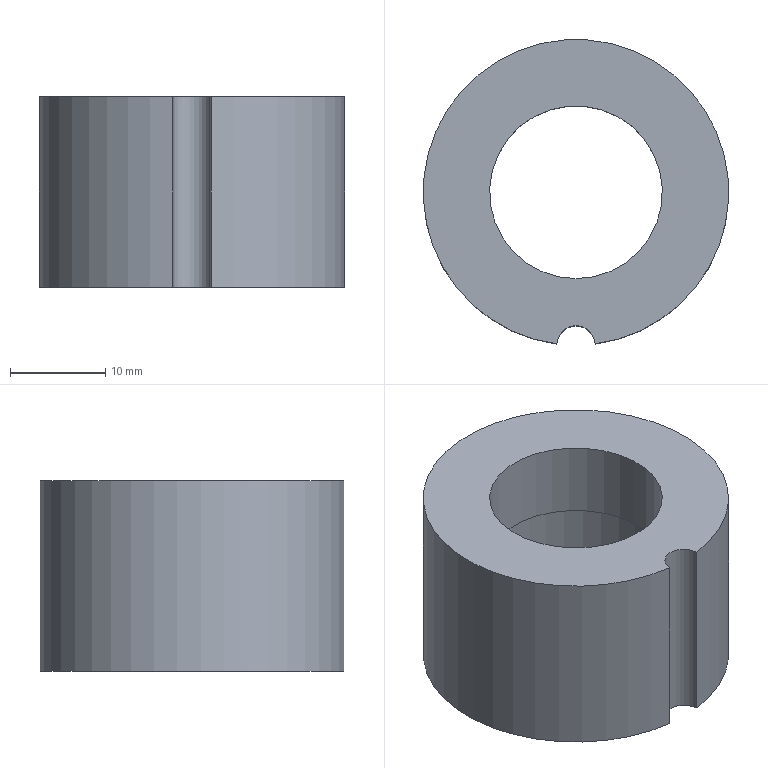Part | NX | features solid 2 | 1 solid | 7 faces | box 32 x 31.875 x 20 mm | volume 9905 mm3 | cylinder 4 | plane 3 | commonest cylinder face diameters 4 x1 18.1 x1 20.6 x1 32 x1
STEP:
#1=CARTESIAN_POINT('',(-688.819,-366.873,17.));
#2=VERTEX_POINT('',#1);
#3=CARTESIAN_POINT('',(-688.819,-366.873,37.));
#4=VERTEX_POINT('',#3);
#5=CARTESIAN_POINT('',(-688.819,-366.873,27.));
#6=DIRECTION('',(0.,0.,1.));
#7=VECTOR('',#6,1000.);
#8=LINE('',#5,#7);
#9=EDGE_CURVE('',#2,#4,#8,.T.);
#10=ORIENTED_EDGE('',*,*,#9,.F.);
#11=CARTESIAN_POINT('',(-692.811,-366.873,17.));
#12=VERTEX_POINT('',#11);
#13=CARTESIAN_POINT('',(-690.815,-350.998,17.));
#14=DIRECTION('',(0.,0.,1.));
#15=DIRECTION('',(0.,-1.,0.));
#16=AXIS2_PLACEMENT_3D('',#13,#14,#15);
#17=CIRCLE('',#16,16.);
#18=EDGE_CURVE('',#2,#12,#17,.T.);
#19=ORIENTED_EDGE('',*,*,#18,.T.);
#20=CARTESIAN_POINT('',(-692.811,-366.873,37.));
#21=VERTEX_POINT('',#20);
#22=CARTESIAN_POINT('',(-692.811,-366.873,27.));
#23=DIRECTION('',(0.,0.,1.));
#24=VECTOR('',#23,1000.);
#25=LINE('',#22,#24);
#26=EDGE_CURVE('',#21,#12,#25,.F.);
#27=ORIENTED_EDGE('',*,*,#26,.F.);
#28=CARTESIAN_POINT('',(-690.815,-350.998,37.));
#29=DIRECTION('',(0.,0.,1.));
#30=DIRECTION('',(0.,-1.,0.));
#31=AXIS2_PLACEMENT_3D('',#28,#29,#30);
#32=CIRCLE('',#31,16.);
#33=EDGE_CURVE('',#4,#21,#32,.T.);
#34=ORIENTED_EDGE('',*,*,#33,.F.);
#35=EDGE_LOOP('',(#10,#19,#27,#34));
#36=FACE_BOUND('',#35,.T.);
#37=CARTESIAN_POINT('',(-690.815,-350.998,17.));
#38=DIRECTION('',(0.,0.,1.));
#39=DIRECTION('',(0.,-1.,0.));
#40=AXIS2_PLACEMENT_3D('',#37,#38,#39);
#41=CYLINDRICAL_SURFACE('',#40,16.);
#42=ADVANCED_FACE('',(#36),#41,.T.);
#43=CARTESIAN_POINT('',(-690.815,-361.298,17.));
#44=VERTEX_POINT('',#43);
#45=CARTESIAN_POINT('',(-690.815,-350.998,17.));
#46=DIRECTION('',(0.,0.,1.));
#47=DIRECTION('',(0.,-1.,0.));
#48=AXIS2_PLACEMENT_3D('',#45,#46,#47);
#49=CIRCLE('',#48,10.3);
#50=EDGE_CURVE('',#44,#44,#49,.T.);
#51=ORIENTED_EDGE('',*,*,#50,.T.);
#52=EDGE_LOOP('',(#51));
#53=FACE_BOUND('',#52,.T.);
#54=ORIENTED_EDGE('',*,*,#18,.F.);
#55=CARTESIAN_POINT('',(-690.815,-366.998,17.));
#56=DIRECTION('',(0.,0.,1.));
#57=DIRECTION('',(0.,-1.,0.));
#58=AXIS2_PLACEMENT_3D('',#55,#56,#57);
#59=CIRCLE('',#58,2.);
#60=EDGE_CURVE('',#2,#12,#59,.T.);
#61=ORIENTED_EDGE('',*,*,#60,.T.);
#62=EDGE_LOOP('',(#54,#61));
#63=FACE_BOUND('',#62,.T.);
#64=CARTESIAN_POINT('',(-690.815,-350.998,17.));
#65=DIRECTION('',(0.,0.,1.));
#66=DIRECTION('',(0.,-1.,0.));
#67=AXIS2_PLACEMENT_3D('',#64,#65,#66);
#68=PLANE('',#67);
#69=ADVANCED_FACE('',(#53,#63),#68,.F.);
#70=CARTESIAN_POINT('',(-690.815,-360.048,37.));
#71=VERTEX_POINT('',#70);
#72=CARTESIAN_POINT('',(-690.815,-350.998,37.));
#73=DIRECTION('',(0.,0.,1.));
#74=DIRECTION('',(0.,-1.,0.));
#75=AXIS2_PLACEMENT_3D('',#72,#73,#74);
#76=CIRCLE('',#75,9.05);
#77=EDGE_CURVE('',#71,#71,#76,.T.);
#78=ORIENTED_EDGE('',*,*,#77,.F.);
#79=EDGE_LOOP('',(#78));
#80=FACE_BOUND('',#79,.T.);
#81=CARTESIAN_POINT('',(-690.815,-366.998,37.));
#82=DIRECTION('',(0.,0.,1.));
#83=DIRECTION('',(0.,-1.,0.));
#84=AXIS2_PLACEMENT_3D('',#81,#82,#83);
#85=CIRCLE('',#84,2.);
#86=EDGE_CURVE('',#4,#21,#85,.T.);
#87=ORIENTED_EDGE('',*,*,#86,.F.);
#88=ORIENTED_EDGE('',*,*,#33,.T.);
#89=EDGE_LOOP('',(#87,#88));
#90=FACE_BOUND('',#89,.T.);
#91=CARTESIAN_POINT('',(-690.815,-350.998,37.));
#92=DIRECTION('',(0.,0.,1.));
#93=DIRECTION('',(0.,-1.,0.));
#94=AXIS2_PLACEMENT_3D('',#91,#92,#93);
#95=PLANE('',#94);
#96=ADVANCED_FACE('',(#80,#90),#95,.T.);
#97=ORIENTED_EDGE('',*,*,#50,.F.);
#98=EDGE_LOOP('',(#97));
#99=FACE_BOUND('',#98,.T.);
#100=CARTESIAN_POINT('',(-690.815,-361.298,29.));
#101=VERTEX_POINT('',#100);
#102=CARTESIAN_POINT('',(-690.815,-350.998,29.));
#103=DIRECTION('',(0.,0.,1.));
#104=DIRECTION('',(0.,-1.,0.));
#105=AXIS2_PLACEMENT_3D('',#102,#103,#104);
#106=CIRCLE('',#105,10.3);
#107=EDGE_CURVE('',#101,#101,#106,.T.);
#108=ORIENTED_EDGE('',*,*,#107,.T.);
#109=EDGE_LOOP('',(#108));
#110=FACE_BOUND('',#109,.T.);
#111=CARTESIAN_POINT('',(-690.815,-350.998,17.));
#112=DIRECTION('',(0.,0.,1.));
#113=DIRECTION('',(0.,-1.,0.));
#114=AXIS2_PLACEMENT_3D('',#111,#112,#113);
#115=CYLINDRICAL_SURFACE('',#114,10.3);
#116=ADVANCED_FACE('',(#99,#110),#115,.F.);
#117=CARTESIAN_POINT('',(-690.815,-360.048,29.));
#118=VERTEX_POINT('',#117);
#119=CARTESIAN_POINT('',(-690.815,-350.998,29.));
#120=DIRECTION('',(0.,0.,1.));
#121=DIRECTION('',(0.,-1.,0.));
#122=AXIS2_PLACEMENT_3D('',#119,#120,#121);
#123=CIRCLE('',#122,9.05);
#124=EDGE_CURVE('',#118,#118,#123,.T.);
#125=ORIENTED_EDGE('',*,*,#124,.T.);
#126=EDGE_LOOP('',(#125));
#127=FACE_BOUND('',#126,.T.);
#128=ORIENTED_EDGE('',*,*,#107,.F.);
#129=EDGE_LOOP('',(#128));
#130=FACE_BOUND('',#129,.T.);
#131=CARTESIAN_POINT('',(-690.815,-350.998,29.));
#132=DIRECTION('',(0.,0.,1.));
#133=DIRECTION('',(0.,-1.,0.));
#134=AXIS2_PLACEMENT_3D('',#131,#132,#133);
#135=PLANE('',#134);
#136=ADVANCED_FACE('',(#127,#130),#135,.F.);
#137=ORIENTED_EDGE('',*,*,#9,.T.);
#138=ORIENTED_EDGE('',*,*,#86,.T.);
#139=ORIENTED_EDGE('',*,*,#26,.T.);
#140=ORIENTED_EDGE('',*,*,#60,.F.);
#141=EDGE_LOOP('',(#137,#138,#139,#140));
#142=FACE_BOUND('',#141,.T.);
#143=CARTESIAN_POINT('',(-690.815,-366.998,17.));
#144=DIRECTION('',(0.,0.,1.));
#145=DIRECTION('',(0.,-1.,0.));
#146=AXIS2_PLACEMENT_3D('',#143,#144,#145);
#147=CYLINDRICAL_SURFACE('',#146,2.);
#148=ADVANCED_FACE('',(#142),#147,.F.);
#149=ORIENTED_EDGE('',*,*,#77,.T.);
#150=EDGE_LOOP('',(#149));
#151=FACE_BOUND('',#150,.T.);
#152=ORIENTED_EDGE('',*,*,#124,.F.);
#153=EDGE_LOOP('',(#152));
#154=FACE_BOUND('',#153,.T.);
#155=CARTESIAN_POINT('',(-690.815,-350.998,17.));
#156=DIRECTION('',(0.,0.,1.));
#157=DIRECTION('',(0.,-1.,0.));
#158=AXIS2_PLACEMENT_3D('',#155,#156,#157);
#159=CYLINDRICAL_SURFACE('',#158,9.05);
#160=ADVANCED_FACE('',(#151,#154),#159,.F.);
#161=CLOSED_SHELL('',(#42,#69,#96,#116,#136,#148,#160));
#162=MANIFOLD_SOLID_BREP('',#161);
#163=(LENGTH_UNIT()NAMED_UNIT(*)SI_UNIT(.MILLI.,.METRE.));
#164=UNCERTAINTY_MEASURE_WITH_UNIT(LENGTH_MEASURE(0.00001),#163,'','');
#165=(NAMED_UNIT(*)PLANE_ANGLE_UNIT()SI_UNIT($,.RADIAN.));
#166=(NAMED_UNIT(*)SI_UNIT($,.STERADIAN.)SOLID_ANGLE_UNIT());
#167=(GEOMETRIC_REPRESENTATION_CONTEXT(3)GLOBAL_UNCERTAINTY_ASSIGNED_CONTEXT((#164))GLOBAL_UNIT_ASSIGNED_CONTEXT((#163,#165,#166))REPRESENTATION_CONTEXT('',''));
#168=ADVANCED_BREP_SHAPE_REPRESENTATION('',(#162),#167);